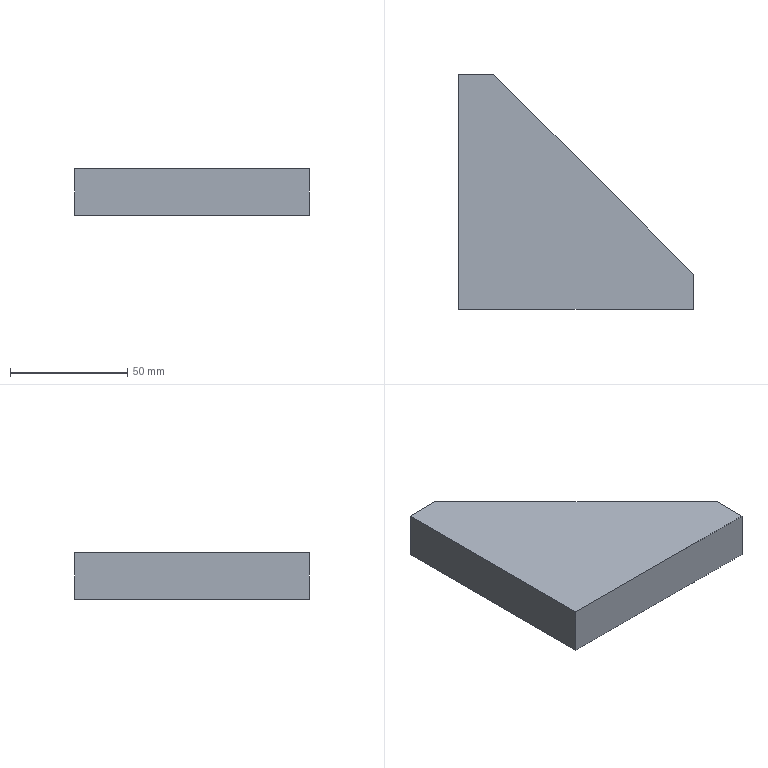Part | SolidWorks | features Extrusion 1 | 1 solid | 7 faces | box 100 x 100 x 20 mm | volume 127750 mm3 | plane 7
STEP:
#1=CARTESIAN_POINT('',(0.,0.,0.));
#2=VERTEX_POINT('',#1);
#3=CARTESIAN_POINT('',(100.,0.,0.));
#4=VERTEX_POINT('',#3);
#5=CARTESIAN_POINT('',(100.,0.,0.));
#6=DIRECTION('',(1.,0.,0.));
#7=VECTOR('',#6,1000.);
#8=LINE('',#5,#7);
#9=EDGE_CURVE('',#2,#4,#8,.T.);
#10=ORIENTED_EDGE('',*,*,#9,.T.);
#11=CARTESIAN_POINT('',(100.,0.,20.));
#12=VERTEX_POINT('',#11);
#13=CARTESIAN_POINT('',(100.,0.,20.));
#14=DIRECTION('',(0.,0.,-1.));
#15=VECTOR('',#14,1000.);
#16=LINE('',#13,#15);
#17=EDGE_CURVE('',#12,#4,#16,.T.);
#18=ORIENTED_EDGE('',*,*,#17,.F.);
#19=CARTESIAN_POINT('',(0.,0.,20.));
#20=VERTEX_POINT('',#19);
#21=CARTESIAN_POINT('',(100.,0.,20.));
#22=DIRECTION('',(1.,0.,0.));
#23=VECTOR('',#22,1000.);
#24=LINE('',#21,#23);
#25=EDGE_CURVE('',#20,#12,#24,.T.);
#26=ORIENTED_EDGE('',*,*,#25,.F.);
#27=CARTESIAN_POINT('',(0.,0.,20.));
#28=DIRECTION('',(0.,0.,-1.));
#29=VECTOR('',#28,1000.);
#30=LINE('',#27,#29);
#31=EDGE_CURVE('',#20,#2,#30,.T.);
#32=ORIENTED_EDGE('',*,*,#31,.T.);
#33=EDGE_LOOP('',(#10,#18,#26,#32));
#34=FACE_OUTER_BOUND('',#33,.T.);
#35=CARTESIAN_POINT('',(100.,0.,20.));
#36=DIRECTION('',(0.,1.,0.));
#37=DIRECTION('',(0.,0.,1.));
#38=AXIS2_PLACEMENT_3D('',#35,#36,#37);
#39=PLANE('',#38);
#40=ADVANCED_FACE('',(#34),#39,.F.);
#41=CARTESIAN_POINT('',(100.,15.,0.));
#42=VERTEX_POINT('',#41);
#43=CARTESIAN_POINT('',(100.,15.,0.));
#44=DIRECTION('',(0.,1.,0.));
#45=VECTOR('',#44,1000.);
#46=LINE('',#43,#45);
#47=EDGE_CURVE('',#4,#42,#46,.T.);
#48=ORIENTED_EDGE('',*,*,#47,.T.);
#49=CARTESIAN_POINT('',(100.,15.,20.));
#50=VERTEX_POINT('',#49);
#51=CARTESIAN_POINT('',(100.,15.,20.));
#52=DIRECTION('',(0.,0.,-1.));
#53=VECTOR('',#52,1000.);
#54=LINE('',#51,#53);
#55=EDGE_CURVE('',#50,#42,#54,.T.);
#56=ORIENTED_EDGE('',*,*,#55,.F.);
#57=CARTESIAN_POINT('',(100.,15.,20.));
#58=DIRECTION('',(0.,1.,0.));
#59=VECTOR('',#58,1000.);
#60=LINE('',#57,#59);
#61=EDGE_CURVE('',#12,#50,#60,.T.);
#62=ORIENTED_EDGE('',*,*,#61,.F.);
#63=ORIENTED_EDGE('',*,*,#17,.T.);
#64=EDGE_LOOP('',(#48,#56,#62,#63));
#65=FACE_OUTER_BOUND('',#64,.T.);
#66=CARTESIAN_POINT('',(100.,15.,20.));
#67=DIRECTION('',(-1.,0.,0.));
#68=DIRECTION('',(0.,0.,1.));
#69=AXIS2_PLACEMENT_3D('',#66,#67,#68);
#70=PLANE('',#69);
#71=ADVANCED_FACE('',(#65),#70,.F.);
#72=CARTESIAN_POINT('',(15.,100.,0.));
#73=VERTEX_POINT('',#72);
#74=CARTESIAN_POINT('',(15.,100.,0.));
#75=DIRECTION('',(-0.7071,0.7071,0.));
#76=VECTOR('',#75,1000.);
#77=LINE('',#74,#76);
#78=EDGE_CURVE('',#42,#73,#77,.T.);
#79=ORIENTED_EDGE('',*,*,#78,.T.);
#80=CARTESIAN_POINT('',(15.,100.,20.));
#81=VERTEX_POINT('',#80);
#82=CARTESIAN_POINT('',(15.,100.,20.));
#83=DIRECTION('',(0.,0.,-1.));
#84=VECTOR('',#83,1000.);
#85=LINE('',#82,#84);
#86=EDGE_CURVE('',#81,#73,#85,.T.);
#87=ORIENTED_EDGE('',*,*,#86,.F.);
#88=CARTESIAN_POINT('',(15.,100.,20.));
#89=DIRECTION('',(-0.7071,0.7071,0.));
#90=VECTOR('',#89,1000.);
#91=LINE('',#88,#90);
#92=EDGE_CURVE('',#50,#81,#91,.T.);
#93=ORIENTED_EDGE('',*,*,#92,.F.);
#94=ORIENTED_EDGE('',*,*,#55,.T.);
#95=EDGE_LOOP('',(#79,#87,#93,#94));
#96=FACE_OUTER_BOUND('',#95,.T.);
#97=CARTESIAN_POINT('',(15.,100.,20.));
#98=DIRECTION('',(-0.7071,-0.7071,0.));
#99=DIRECTION('',(0.7071,-0.7071,0.));
#100=AXIS2_PLACEMENT_3D('',#97,#98,#99);
#101=PLANE('',#100);
#102=ADVANCED_FACE('',(#96),#101,.F.);
#103=CARTESIAN_POINT('',(0.,100.,0.));
#104=VERTEX_POINT('',#103);
#105=CARTESIAN_POINT('',(0.,100.,0.));
#106=DIRECTION('',(-1.,0.,0.));
#107=VECTOR('',#106,1000.);
#108=LINE('',#105,#107);
#109=EDGE_CURVE('',#73,#104,#108,.T.);
#110=ORIENTED_EDGE('',*,*,#109,.T.);
#111=CARTESIAN_POINT('',(0.,100.,20.));
#112=VERTEX_POINT('',#111);
#113=CARTESIAN_POINT('',(0.,100.,20.));
#114=DIRECTION('',(0.,0.,-1.));
#115=VECTOR('',#114,1000.);
#116=LINE('',#113,#115);
#117=EDGE_CURVE('',#112,#104,#116,.T.);
#118=ORIENTED_EDGE('',*,*,#117,.F.);
#119=CARTESIAN_POINT('',(0.,100.,20.));
#120=DIRECTION('',(-1.,0.,0.));
#121=VECTOR('',#120,1000.);
#122=LINE('',#119,#121);
#123=EDGE_CURVE('',#81,#112,#122,.T.);
#124=ORIENTED_EDGE('',*,*,#123,.F.);
#125=ORIENTED_EDGE('',*,*,#86,.T.);
#126=EDGE_LOOP('',(#110,#118,#124,#125));
#127=FACE_OUTER_BOUND('',#126,.T.);
#128=CARTESIAN_POINT('',(0.,100.,20.));
#129=DIRECTION('',(0.,-1.,0.));
#130=DIRECTION('',(0.,0.,-1.));
#131=AXIS2_PLACEMENT_3D('',#128,#129,#130);
#132=PLANE('',#131);
#133=ADVANCED_FACE('',(#127),#132,.F.);
#134=CARTESIAN_POINT('',(0.,0.,0.));
#135=DIRECTION('',(0.,-1.,0.));
#136=VECTOR('',#135,1000.);
#137=LINE('',#134,#136);
#138=EDGE_CURVE('',#104,#2,#137,.T.);
#139=ORIENTED_EDGE('',*,*,#138,.T.);
#140=ORIENTED_EDGE('',*,*,#31,.F.);
#141=CARTESIAN_POINT('',(0.,0.,20.));
#142=DIRECTION('',(0.,-1.,0.));
#143=VECTOR('',#142,1000.);
#144=LINE('',#141,#143);
#145=EDGE_CURVE('',#112,#20,#144,.T.);
#146=ORIENTED_EDGE('',*,*,#145,.F.);
#147=ORIENTED_EDGE('',*,*,#117,.T.);
#148=EDGE_LOOP('',(#139,#140,#146,#147));
#149=FACE_OUTER_BOUND('',#148,.T.);
#150=CARTESIAN_POINT('',(0.,0.,20.));
#151=DIRECTION('',(1.,0.,0.));
#152=DIRECTION('',(0.,0.,-1.));
#153=AXIS2_PLACEMENT_3D('',#150,#151,#152);
#154=PLANE('',#153);
#155=ADVANCED_FACE('',(#149),#154,.F.);
#156=ORIENTED_EDGE('',*,*,#25,.T.);
#157=ORIENTED_EDGE('',*,*,#61,.T.);
#158=ORIENTED_EDGE('',*,*,#92,.T.);
#159=ORIENTED_EDGE('',*,*,#123,.T.);
#160=ORIENTED_EDGE('',*,*,#145,.T.);
#161=EDGE_LOOP('',(#156,#157,#158,#159,#160));
#162=FACE_OUTER_BOUND('',#161,.T.);
#163=CARTESIAN_POINT('',(0.,0.,20.));
#164=DIRECTION('',(0.,0.,-1.));
#165=DIRECTION('',(-1.,0.,0.));
#166=AXIS2_PLACEMENT_3D('',#163,#164,#165);
#167=PLANE('',#166);
#168=ADVANCED_FACE('',(#162),#167,.F.);
#169=ORIENTED_EDGE('',*,*,#9,.F.);
#170=ORIENTED_EDGE('',*,*,#138,.F.);
#171=ORIENTED_EDGE('',*,*,#109,.F.);
#172=ORIENTED_EDGE('',*,*,#78,.F.);
#173=ORIENTED_EDGE('',*,*,#47,.F.);
#174=EDGE_LOOP('',(#169,#170,#171,#172,#173));
#175=FACE_OUTER_BOUND('',#174,.T.);
#176=CARTESIAN_POINT('',(0.,0.,0.));
#177=DIRECTION('',(0.,0.,-1.));
#178=DIRECTION('',(-1.,0.,0.));
#179=AXIS2_PLACEMENT_3D('',#176,#177,#178);
#180=PLANE('',#179);
#181=ADVANCED_FACE('',(#175),#180,.T.);
#182=CLOSED_SHELL('',(#40,#71,#102,#133,#155,#168,#181));
#183=MANIFOLD_SOLID_BREP('',#182);
#184=CARTESIAN_POINT('',(0.,0.,0.));
#185=DIRECTION('',(0.,0.,1.));
#186=DIRECTION('',(1.,0.,0.));
#187=AXIS2_PLACEMENT_3D('',#184,#185,#186);
#188=(LENGTH_UNIT()NAMED_UNIT(*)SI_UNIT(.MILLI.,.METRE.));
#189=UNCERTAINTY_MEASURE_WITH_UNIT(LENGTH_MEASURE(0.00001),#188,'','');
#190=(NAMED_UNIT(*)PLANE_ANGLE_UNIT()SI_UNIT($,.RADIAN.));
#191=(NAMED_UNIT(*)SI_UNIT($,.STERADIAN.)SOLID_ANGLE_UNIT());
#192=(GEOMETRIC_REPRESENTATION_CONTEXT(3)GLOBAL_UNCERTAINTY_ASSIGNED_CONTEXT((#189))GLOBAL_UNIT_ASSIGNED_CONTEXT((#188,#190,#191))REPRESENTATION_CONTEXT('',''));
#193=ADVANCED_BREP_SHAPE_REPRESENTATION('',(#183,#187),#192);